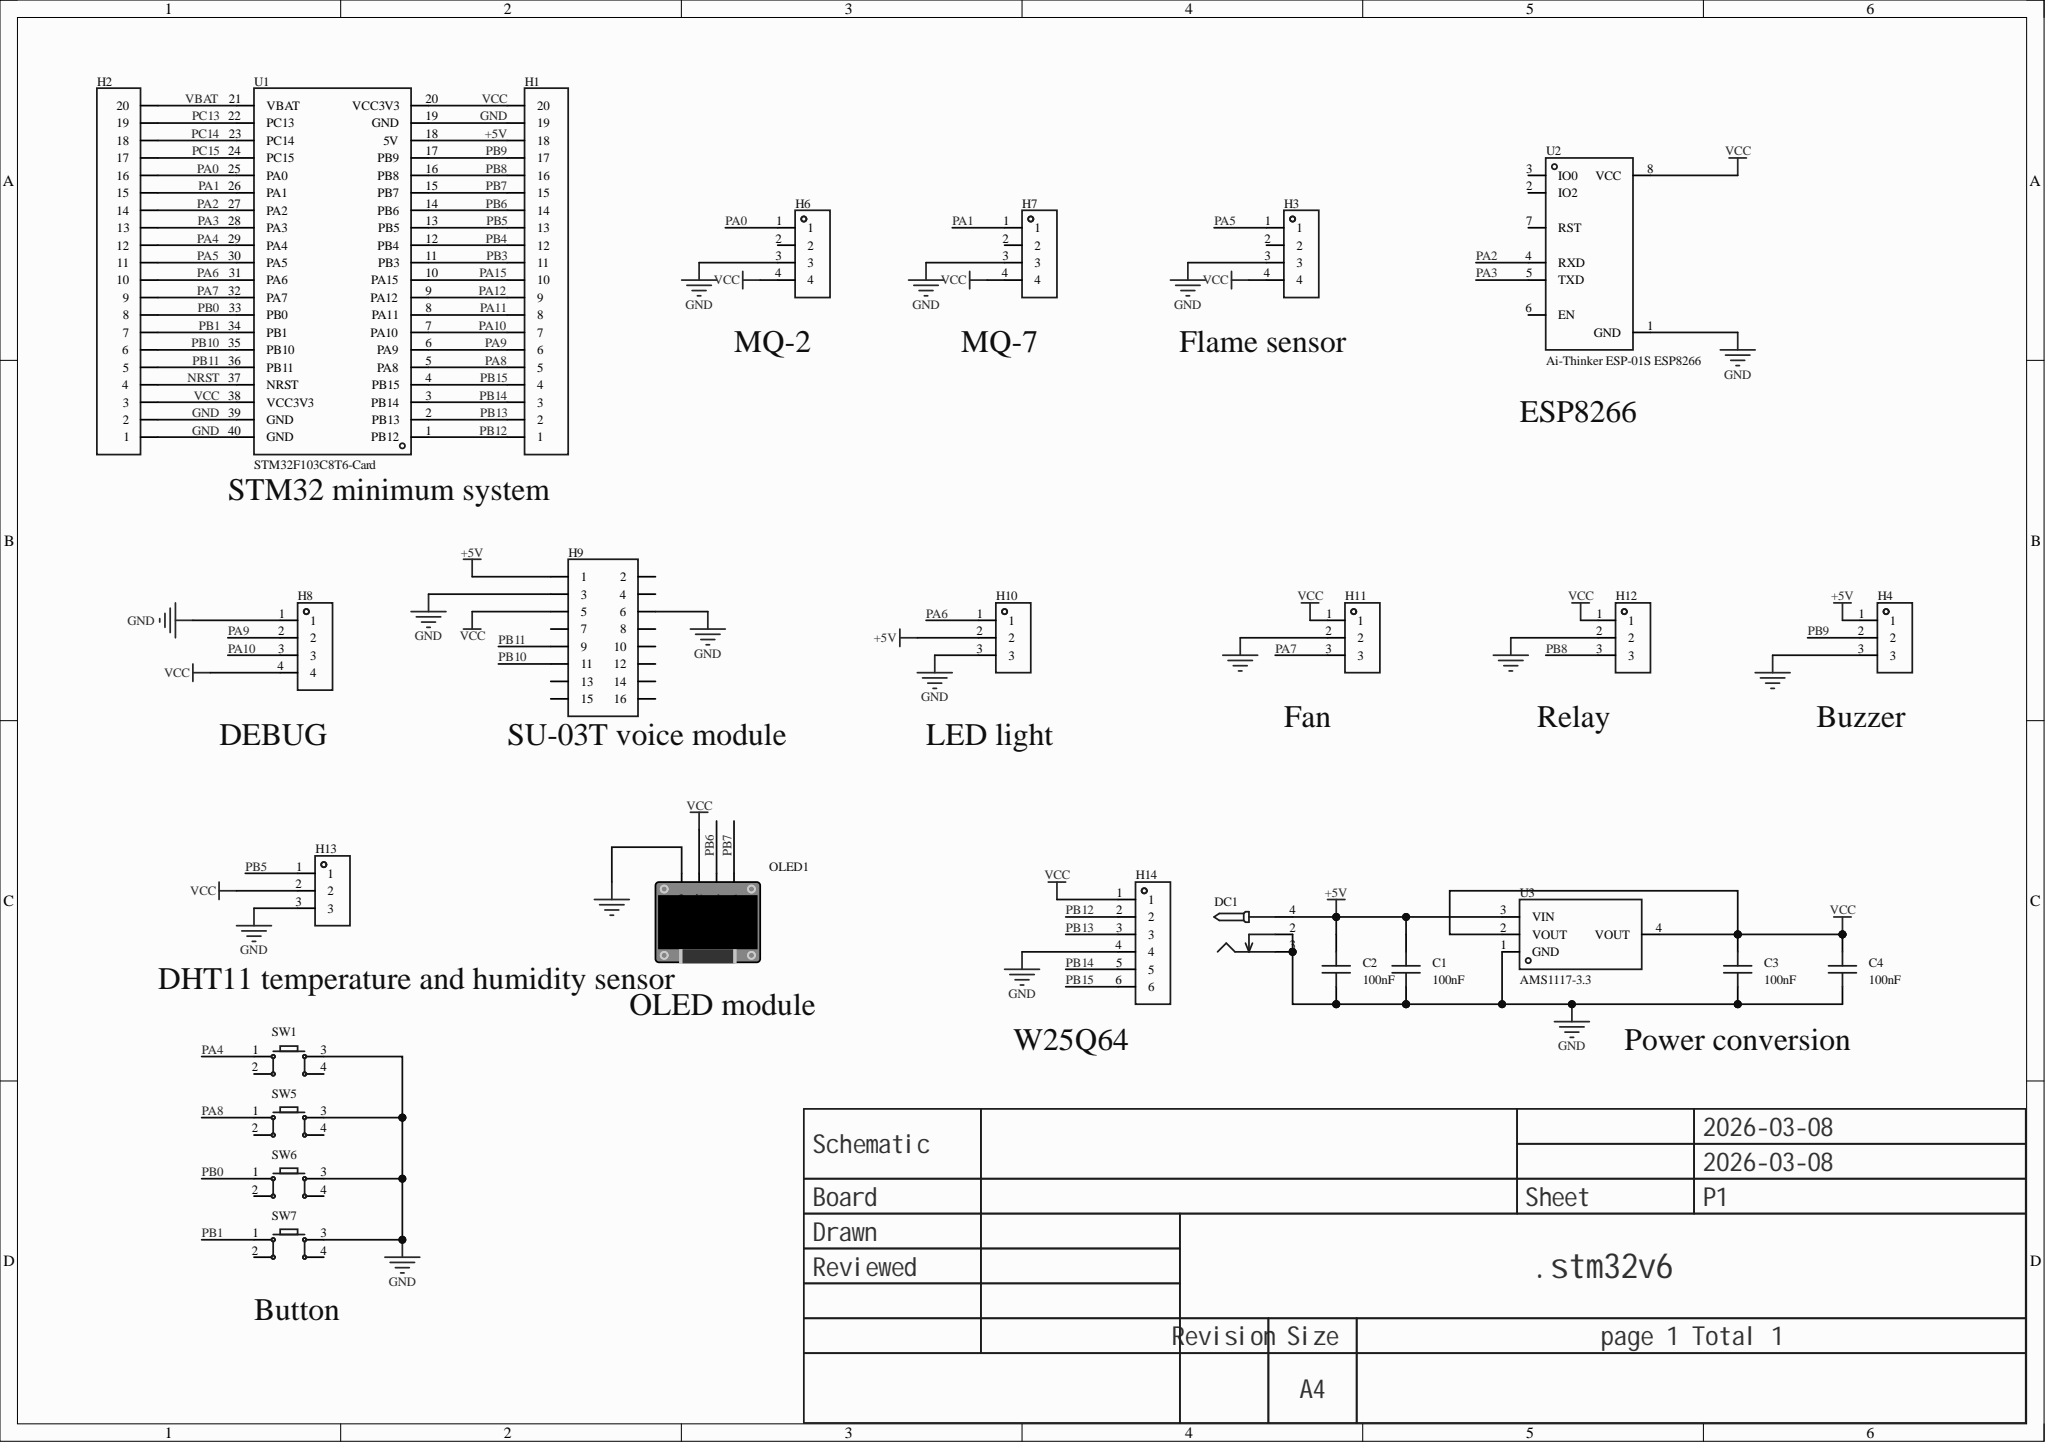Circuit board | Altium Designer | 26 parts | 37 nets
Bill of materials:
Comment,Description,Designator,Footprint,LibRef,Quantity
"100nF","","C1, C2, C3, C4","C0603","CAP_0603","4"
"","","DC1","DC-2.0","DC-005_2.0","1"
"","","H1, H2","HDR-TH_20P-P2.54-V-F","HDR-F_2.54_1x20P","2"
"","","H3, H6, H7, H8","HDR-TH_4P-P2.54-V-F","HDR-F_2.54_1x4P","4"
"","","H4, H10, H11, H12, H13","HDR-TH_3P-P2.54-V-F","HDR-F_2.54_1x3P","5"
"","","H9","HDR-TH_16P-P2.54-V-M-R2-C8-S2.54","HDR-M_2.54_2x8","1"
"","","H14","HDR-TH_6P-P2.54-V-F","HDR-F_2.54_1x6P","1"
"","","OLED1","0.96OLED_4P","0.96OLED模块_4P","1"
"","","SW1, SW5, SW6, SW7","SW-TH_4P-L6.0-W6.0-P4.50-LS6.5","Key_TH_6x6x6","4"
"STM32F103C8T6-Card","","U1","CONN-TH_L53.3-W22.9_STM32F103C8T6-CARD","STM32F103C8T6-Card","1"
"Ai-Thinker ESP-01S ESP8266","","U2","WIFIM-TH_8P-L24.7-W14.4-P2.54","Ai-Thinker ESP-01S ESP8266","1"
"AMS1117-3.3","Output type: fixed; operating voltage: -; output voltage: 3.3V; output current: 1A; ripple rejection (PSRR): 72dB@(120Hz); output polarity: positive;","U3","SOT-223-3_L6.5-W3.4-P2.30-LS7.0-BR","AMS1117-3.3_C6186","1"
Netlist (Protel format):
[
C1
C0603
100nF



]
[
C2
C0603
100nF



]
[
C3
C0603
100nF



]
[
C4
C0603
100nF



]
[
DC1
DC-2.0




]
[
H1
HDR-TH_20P-P2.54-V-F




]
[
H2
HDR-TH_20P-P2.54-V-F




]
[
H3
HDR-TH_4P-P2.54-V-F




]
[
H4
HDR-TH_3P-P2.54-V-F




]
[
H6
HDR-TH_4P-P2.54-V-F




]
[
H7
HDR-TH_4P-P2.54-V-F




]
[
H8
HDR-TH_4P-P2.54-V-F




]
[
H9
HDR-TH_16P-P2.54-V-M-R2-C8-S2.54




]
[
H10
HDR-TH_3P-P2.54-V-F




]
[
H11
HDR-TH_3P-P2.54-V-F




]
[
H12
HDR-TH_3P-P2.54-V-F




]
[
H13
HDR-TH_3P-P2.54-V-F




]
[
H14
HDR-TH_6P-P2.54-V-F




]
[
OLED1
0.96OLED_4P




]
[
SW1
SW-TH_4P-L6.0-W6.0-P4.50-LS6.5




]
[
SW5
SW-TH_4P-L6.0-W6.0-P4.50-LS6.5




]
[
SW6
SW-TH_4P-L6.0-W6.0-P4.50-LS6.5




]
[
SW7
SW-TH_4P-L6.0-W6.0-P4.50-LS6.5




]
[
U1
CONN-TH_L53.3-W22.9_STM32F103C8T6-CARD
STM32F103C8T6-Card



]
[
U2
WIFIM-TH_8P-L24.7-W14.4-P2.54
Ai-Thinker ESP-01S ESP8266



]
[
U3
SOT-223-3_L6.5-W3.4-P2.30-LS7.0-BR
AMS1117-3.3



]
(
VCC
C3-2
C4-2
H1-20
H2-3
H3-4
H6-4
H7-4
H8-4
H9-5
H11-1
H12-1
H13-2
H14-1
OLED1-2
U1-20
U1-38
U2-8
U3-2
U3-4
)
(
VBAT
H2-20
U1-21
)
(
PC15
H2-17
U1-24
)
(
PC14
H2-18
U1-23
)
(
PC13
H2-19
U1-22
)
(
PB15
H1-4
H14-6
U1-4
)
(
PB14
H1-3
H14-5
U1-3
)
(
PB13
H1-2
H14-3
U1-2
)
(
PB12
H1-1
H14-2
U1-1
)
(
PB11
H2-5
H9-9
U1-36
)
(
PB10
H2-6
H9-11
U1-35
)
(
PB9
H1-17
H4-2
U1-17
)
(
PB8
H1-16
H12-3
U1-16
)
(
PB7
H1-15
OLED1-4
U1-15
)
(
PB6
H1-14
OLED1-3
U1-14
)
(
PB5
H1-13
H13-1
U1-13
)
(
PB4
H1-12
U1-12
)
(
PB3
H1-11
U1-11
)
(
PB1
H2-7
SW7-1
U1-34
)
(
PB0
H2-8
SW6-1
U1-33
)
(
PA15
H1-10
U1-10
)
(
PA12
H1-9
U1-9
)
(
PA11
H1-8
U1-8
)
(
PA10
H1-7
H8-3
U1-7
)
(
PA9
H1-6
H8-2
U1-6
)
(
PA8
H1-5
SW5-1
U1-5
)
(
PA7
H2-9
H11-3
U1-32
)
(
PA6
H2-10
H10-1
U1-31
)
(
PA5
H2-11
H3-1
U1-30
)
(
PA4
H2-12
SW1-1
U1-29
)
(
PA3
H2-13
U1-28
U2-5
)
(
PA2
H2-14
U1-27
U2-4
)
(
PA1
H2-15
H7-1
U1-26
)
(
PA0
H2-16
H6-1
U1-25
)
(
NRST
H2-4
U1-37
)
(
GND
C1-1
C2-1
C3-1
C4-1
DC1-2
DC1-3
H1-19
H2-1
H2-2
H3-3
H4-3
H6-3
H7-3
H8-1
H9-3
H9-6
H10-3
H11-2
H12-2
H13-3
H14-4
OLED1-1
SW1-3
SW5-3
SW6-3
SW7-3
U1-19
U1-39
U1-40
U2-1
U3-1
)
(
+5V
C1-2
C2-2
DC1-4
H1-18
H4-1
H9-1
H10-2
U1-18
U3-3
)